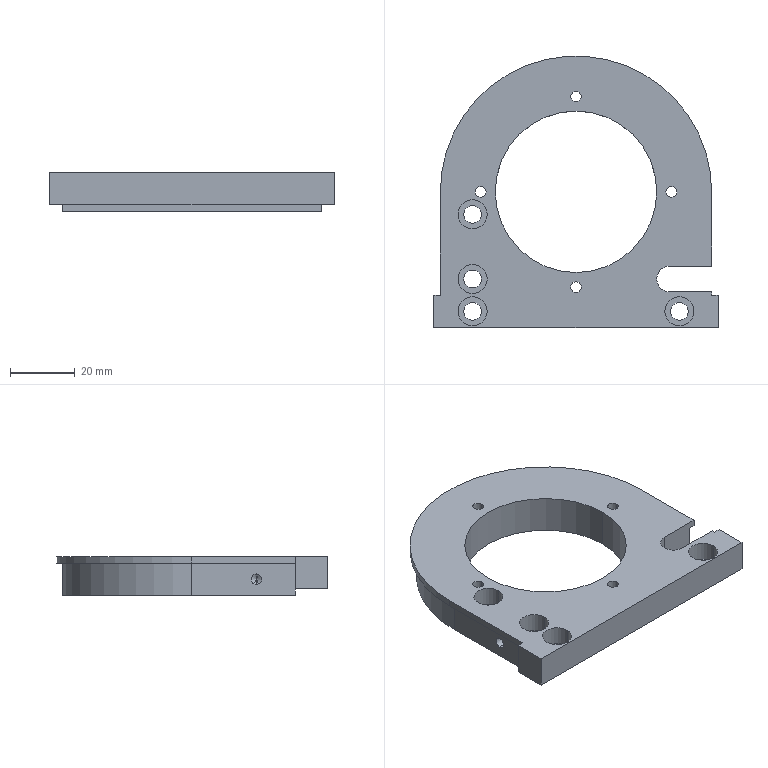Part | SolidWorks | features ICE 6, 3DProfileFeature 3, HoleWzd 3, Extrusion 1, MoveFace 1 | 1 solid | 65 faces | box 88 x 84 x 12 mm | volume 42695 mm3 | cylinder 36 | plane 25 | cone 4 | commonest cylinder face diameters 3.3 x12 5.5 x8 9 x8 2 x2 8 x2 50 x2